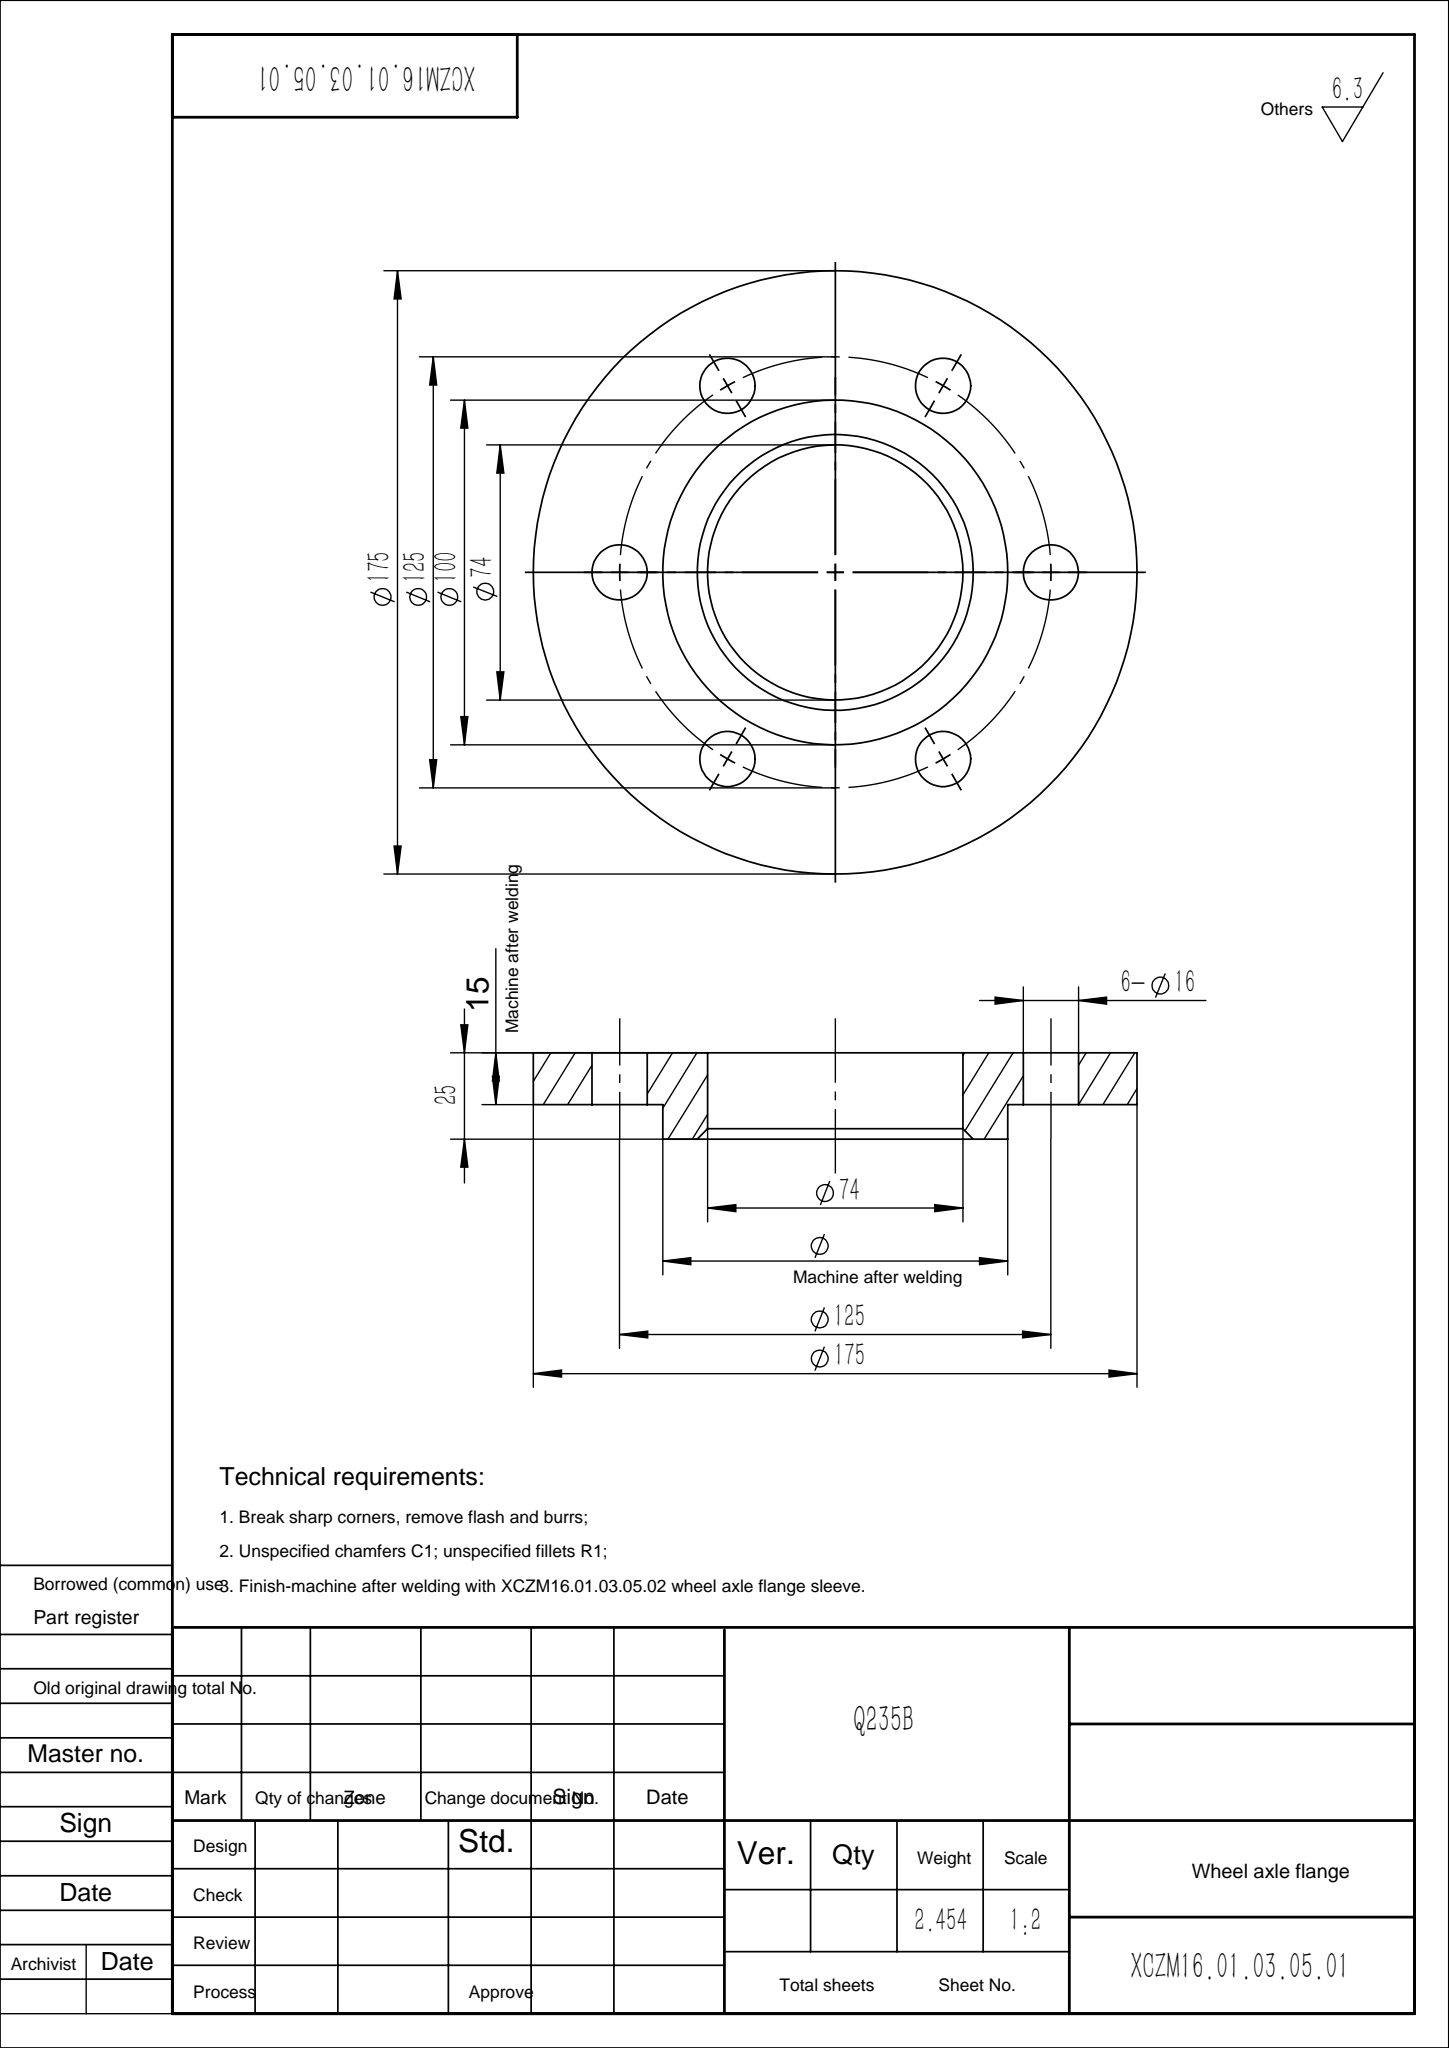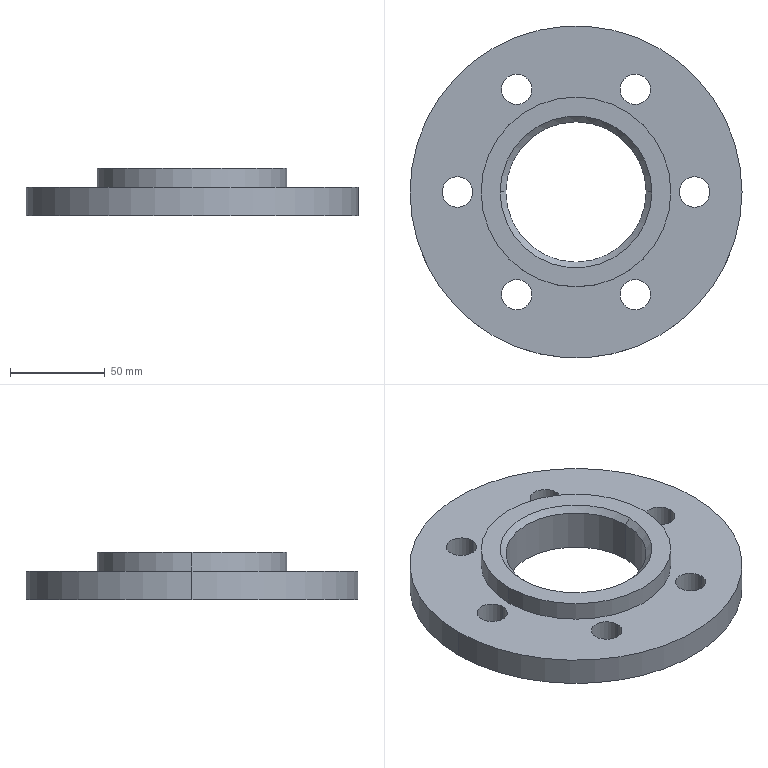Part | SolidWorks | features ICE 2, Chamfer 1, Extrusion 1, HoleWzd 1 | 1 solid | 23 faces | box 175 x 175 x 25 mm | volume 312641 mm3 | cylinder 18 | plane 3 | cone 2 | commonest cylinder face diameters 16 x12 74 x2 100 x2 175 x2
STEP:
#1=CARTESIAN_POINT('',(-37.,0.,7.));
#2=VERTEX_POINT('',#1);
#3=CARTESIAN_POINT('',(37.,0.,7.));
#4=VERTEX_POINT('',#3);
#5=CARTESIAN_POINT('',(0.,0.,7.));
#6=DIRECTION('',(0.,0.,1.));
#7=DIRECTION('',(1.,0.,0.));
#8=AXIS2_PLACEMENT_3D('',#5,#6,#7);
#9=CIRCLE('',#8,37.);
#10=EDGE_CURVE('',#2,#4,#9,.T.);
#11=ORIENTED_EDGE('',*,*,#10,.F.);
#12=CARTESIAN_POINT('',(-40.,0.,10.));
#13=VERTEX_POINT('',#12);
#14=CARTESIAN_POINT('',(-37.,0.,7.));
#15=DIRECTION('',(-0.7071,0.,0.7071));
#16=VECTOR('',#15,1000.);
#17=LINE('',#14,#16);
#18=EDGE_CURVE('',#2,#13,#17,.T.);
#19=ORIENTED_EDGE('',*,*,#18,.T.);
#20=CARTESIAN_POINT('',(40.,0.,10.));
#21=VERTEX_POINT('',#20);
#22=CARTESIAN_POINT('',(0.,0.,10.));
#23=DIRECTION('',(0.,0.,-1.));
#24=DIRECTION('',(1.,0.,0.));
#25=AXIS2_PLACEMENT_3D('',#22,#23,#24);
#26=CIRCLE('',#25,40.);
#27=EDGE_CURVE('',#21,#13,#26,.T.);
#28=ORIENTED_EDGE('',*,*,#27,.F.);
#29=CARTESIAN_POINT('',(37.,0.,7.));
#30=DIRECTION('',(0.7071,0.,0.7071));
#31=VECTOR('',#30,1000.);
#32=LINE('',#29,#31);
#33=EDGE_CURVE('',#4,#21,#32,.T.);
#34=ORIENTED_EDGE('',*,*,#33,.F.);
#35=EDGE_LOOP('',(#11,#19,#28,#34));
#36=FACE_OUTER_BOUND('',#35,.T.);
#37=CARTESIAN_POINT('',(0.,0.,7.));
#38=DIRECTION('',(0.,0.,1.));
#39=DIRECTION('',(1.,0.,0.));
#40=AXIS2_PLACEMENT_3D('',#37,#38,#39);
#41=CONICAL_SURFACE('',#40,37.,0.7854);
#42=ADVANCED_FACE('',(#36),#41,.F.);
#43=CARTESIAN_POINT('',(54.5,0.,-15.));
#44=VERTEX_POINT('',#43);
#45=CARTESIAN_POINT('',(70.5,0.,-15.));
#46=VERTEX_POINT('',#45);
#47=CARTESIAN_POINT('',(62.5,0.,-15.));
#48=DIRECTION('',(0.,0.,1.));
#49=DIRECTION('',(1.,0.,0.));
#50=AXIS2_PLACEMENT_3D('',#47,#48,#49);
#51=CIRCLE('',#50,8.);
#52=EDGE_CURVE('',#44,#46,#51,.T.);
#53=ORIENTED_EDGE('',*,*,#52,.F.);
#54=CARTESIAN_POINT('',(54.5,0.,0.));
#55=VERTEX_POINT('',#54);
#56=CARTESIAN_POINT('',(54.5,0.,0.));
#57=DIRECTION('',(0.,0.,1.));
#58=VECTOR('',#57,1000.);
#59=LINE('',#56,#58);
#60=EDGE_CURVE('',#44,#55,#59,.T.);
#61=ORIENTED_EDGE('',*,*,#60,.T.);
#62=CARTESIAN_POINT('',(70.5,0.,0.));
#63=VERTEX_POINT('',#62);
#64=CARTESIAN_POINT('',(62.5,0.,0.));
#65=DIRECTION('',(0.,0.,1.));
#66=DIRECTION('',(1.,0.,0.));
#67=AXIS2_PLACEMENT_3D('',#64,#65,#66);
#68=CIRCLE('',#67,8.);
#69=EDGE_CURVE('',#55,#63,#68,.T.);
#70=ORIENTED_EDGE('',*,*,#69,.T.);
#71=CARTESIAN_POINT('',(70.5,0.,0.));
#72=DIRECTION('',(0.,0.,1.));
#73=VECTOR('',#72,1000.);
#74=LINE('',#71,#73);
#75=EDGE_CURVE('',#46,#63,#74,.T.);
#76=ORIENTED_EDGE('',*,*,#75,.F.);
#77=EDGE_LOOP('',(#53,#61,#70,#76));
#78=FACE_OUTER_BOUND('',#77,.T.);
#79=CARTESIAN_POINT('',(62.5,0.,0.));
#80=DIRECTION('',(0.,0.,1.));
#81=DIRECTION('',(1.,0.,0.));
#82=AXIS2_PLACEMENT_3D('',#79,#80,#81);
#83=CYLINDRICAL_SURFACE('',#82,8.);
#84=ADVANCED_FACE('',(#78),#83,.F.);
#85=CARTESIAN_POINT('',(23.25,-54.127,-15.));
#86=VERTEX_POINT('',#85);
#87=CARTESIAN_POINT('',(39.25,-54.127,-15.));
#88=VERTEX_POINT('',#87);
#89=CARTESIAN_POINT('',(31.25,-54.127,-15.));
#90=DIRECTION('',(0.,0.,1.));
#91=DIRECTION('',(1.,0.,0.));
#92=AXIS2_PLACEMENT_3D('',#89,#90,#91);
#93=CIRCLE('',#92,8.);
#94=EDGE_CURVE('',#86,#88,#93,.T.);
#95=ORIENTED_EDGE('',*,*,#94,.F.);
#96=CARTESIAN_POINT('',(23.25,-54.127,0.));
#97=VERTEX_POINT('',#96);
#98=CARTESIAN_POINT('',(23.25,-54.127,0.));
#99=DIRECTION('',(0.,0.,1.));
#100=VECTOR('',#99,1000.);
#101=LINE('',#98,#100);
#102=EDGE_CURVE('',#86,#97,#101,.T.);
#103=ORIENTED_EDGE('',*,*,#102,.T.);
#104=CARTESIAN_POINT('',(39.25,-54.127,0.));
#105=VERTEX_POINT('',#104);
#106=CARTESIAN_POINT('',(31.25,-54.127,0.));
#107=DIRECTION('',(0.,0.,1.));
#108=DIRECTION('',(1.,0.,0.));
#109=AXIS2_PLACEMENT_3D('',#106,#107,#108);
#110=CIRCLE('',#109,8.);
#111=EDGE_CURVE('',#97,#105,#110,.T.);
#112=ORIENTED_EDGE('',*,*,#111,.T.);
#113=CARTESIAN_POINT('',(39.25,-54.127,0.));
#114=DIRECTION('',(0.,0.,1.));
#115=VECTOR('',#114,1000.);
#116=LINE('',#113,#115);
#117=EDGE_CURVE('',#88,#105,#116,.T.);
#118=ORIENTED_EDGE('',*,*,#117,.F.);
#119=EDGE_LOOP('',(#95,#103,#112,#118));
#120=FACE_OUTER_BOUND('',#119,.T.);
#121=CARTESIAN_POINT('',(31.25,-54.127,0.));
#122=DIRECTION('',(0.,0.,1.));
#123=DIRECTION('',(1.,0.,0.));
#124=AXIS2_PLACEMENT_3D('',#121,#122,#123);
#125=CYLINDRICAL_SURFACE('',#124,8.);
#126=ADVANCED_FACE('',(#120),#125,.F.);
#127=CARTESIAN_POINT('',(-39.25,-54.127,-15.));
#128=VERTEX_POINT('',#127);
#129=CARTESIAN_POINT('',(-23.25,-54.127,-15.));
#130=VERTEX_POINT('',#129);
#131=CARTESIAN_POINT('',(-31.25,-54.127,-15.));
#132=DIRECTION('',(0.,0.,1.));
#133=DIRECTION('',(1.,0.,0.));
#134=AXIS2_PLACEMENT_3D('',#131,#132,#133);
#135=CIRCLE('',#134,8.);
#136=EDGE_CURVE('',#128,#130,#135,.T.);
#137=ORIENTED_EDGE('',*,*,#136,.F.);
#138=CARTESIAN_POINT('',(-39.25,-54.127,0.));
#139=VERTEX_POINT('',#138);
#140=CARTESIAN_POINT('',(-39.25,-54.127,0.));
#141=DIRECTION('',(0.,0.,1.));
#142=VECTOR('',#141,1000.);
#143=LINE('',#140,#142);
#144=EDGE_CURVE('',#128,#139,#143,.T.);
#145=ORIENTED_EDGE('',*,*,#144,.T.);
#146=CARTESIAN_POINT('',(-23.25,-54.127,0.));
#147=VERTEX_POINT('',#146);
#148=CARTESIAN_POINT('',(-31.25,-54.127,0.));
#149=DIRECTION('',(0.,0.,1.));
#150=DIRECTION('',(1.,0.,0.));
#151=AXIS2_PLACEMENT_3D('',#148,#149,#150);
#152=CIRCLE('',#151,8.);
#153=EDGE_CURVE('',#139,#147,#152,.T.);
#154=ORIENTED_EDGE('',*,*,#153,.T.);
#155=CARTESIAN_POINT('',(-23.25,-54.127,0.));
#156=DIRECTION('',(0.,0.,1.));
#157=VECTOR('',#156,1000.);
#158=LINE('',#155,#157);
#159=EDGE_CURVE('',#130,#147,#158,.T.);
#160=ORIENTED_EDGE('',*,*,#159,.F.);
#161=EDGE_LOOP('',(#137,#145,#154,#160));
#162=FACE_OUTER_BOUND('',#161,.T.);
#163=CARTESIAN_POINT('',(-31.25,-54.127,0.));
#164=DIRECTION('',(0.,0.,1.));
#165=DIRECTION('',(1.,0.,0.));
#166=AXIS2_PLACEMENT_3D('',#163,#164,#165);
#167=CYLINDRICAL_SURFACE('',#166,8.);
#168=ADVANCED_FACE('',(#162),#167,.F.);
#169=CARTESIAN_POINT('',(-70.5,0.,-15.));
#170=VERTEX_POINT('',#169);
#171=CARTESIAN_POINT('',(-54.5,0.,-15.));
#172=VERTEX_POINT('',#171);
#173=CARTESIAN_POINT('',(-62.5,0.,-15.));
#174=DIRECTION('',(0.,0.,1.));
#175=DIRECTION('',(1.,0.,0.));
#176=AXIS2_PLACEMENT_3D('',#173,#174,#175);
#177=CIRCLE('',#176,8.);
#178=EDGE_CURVE('',#170,#172,#177,.T.);
#179=ORIENTED_EDGE('',*,*,#178,.F.);
#180=CARTESIAN_POINT('',(-70.5,0.,0.));
#181=VERTEX_POINT('',#180);
#182=CARTESIAN_POINT('',(-70.5,0.,0.));
#183=DIRECTION('',(0.,0.,1.));
#184=VECTOR('',#183,1000.);
#185=LINE('',#182,#184);
#186=EDGE_CURVE('',#170,#181,#185,.T.);
#187=ORIENTED_EDGE('',*,*,#186,.T.);
#188=CARTESIAN_POINT('',(-54.5,0.,0.));
#189=VERTEX_POINT('',#188);
#190=CARTESIAN_POINT('',(-62.5,0.,0.));
#191=DIRECTION('',(0.,0.,1.));
#192=DIRECTION('',(1.,0.,0.));
#193=AXIS2_PLACEMENT_3D('',#190,#191,#192);
#194=CIRCLE('',#193,8.);
#195=EDGE_CURVE('',#181,#189,#194,.T.);
#196=ORIENTED_EDGE('',*,*,#195,.T.);
#197=CARTESIAN_POINT('',(-54.5,0.,0.));
#198=DIRECTION('',(0.,0.,1.));
#199=VECTOR('',#198,1000.);
#200=LINE('',#197,#199);
#201=EDGE_CURVE('',#172,#189,#200,.T.);
#202=ORIENTED_EDGE('',*,*,#201,.F.);
#203=EDGE_LOOP('',(#179,#187,#196,#202));
#204=FACE_OUTER_BOUND('',#203,.T.);
#205=CARTESIAN_POINT('',(-62.5,0.,0.));
#206=DIRECTION('',(0.,0.,1.));
#207=DIRECTION('',(1.,0.,0.));
#208=AXIS2_PLACEMENT_3D('',#205,#206,#207);
#209=CYLINDRICAL_SURFACE('',#208,8.);
#210=ADVANCED_FACE('',(#204),#209,.F.);
#211=CARTESIAN_POINT('',(-39.25,54.127,-15.));
#212=VERTEX_POINT('',#211);
#213=CARTESIAN_POINT('',(-23.25,54.127,-15.));
#214=VERTEX_POINT('',#213);
#215=CARTESIAN_POINT('',(-31.25,54.127,-15.));
#216=DIRECTION('',(0.,0.,1.));
#217=DIRECTION('',(1.,0.,0.));
#218=AXIS2_PLACEMENT_3D('',#215,#216,#217);
#219=CIRCLE('',#218,8.);
#220=EDGE_CURVE('',#212,#214,#219,.T.);
#221=ORIENTED_EDGE('',*,*,#220,.F.);
#222=CARTESIAN_POINT('',(-39.25,54.127,0.));
#223=VERTEX_POINT('',#222);
#224=CARTESIAN_POINT('',(-39.25,54.127,0.));
#225=DIRECTION('',(0.,0.,1.));
#226=VECTOR('',#225,1000.);
#227=LINE('',#224,#226);
#228=EDGE_CURVE('',#212,#223,#227,.T.);
#229=ORIENTED_EDGE('',*,*,#228,.T.);
#230=CARTESIAN_POINT('',(-23.25,54.127,0.));
#231=VERTEX_POINT('',#230);
#232=CARTESIAN_POINT('',(-31.25,54.127,0.));
#233=DIRECTION('',(0.,0.,1.));
#234=DIRECTION('',(1.,0.,0.));
#235=AXIS2_PLACEMENT_3D('',#232,#233,#234);
#236=CIRCLE('',#235,8.);
#237=EDGE_CURVE('',#223,#231,#236,.T.);
#238=ORIENTED_EDGE('',*,*,#237,.T.);
#239=CARTESIAN_POINT('',(-23.25,54.127,0.));
#240=DIRECTION('',(0.,0.,1.));
#241=VECTOR('',#240,1000.);
#242=LINE('',#239,#241);
#243=EDGE_CURVE('',#214,#231,#242,.T.);
#244=ORIENTED_EDGE('',*,*,#243,.F.);
#245=EDGE_LOOP('',(#221,#229,#238,#244));
#246=FACE_OUTER_BOUND('',#245,.T.);
#247=CARTESIAN_POINT('',(-31.25,54.127,0.));
#248=DIRECTION('',(0.,0.,1.));
#249=DIRECTION('',(1.,0.,0.));
#250=AXIS2_PLACEMENT_3D('',#247,#248,#249);
#251=CYLINDRICAL_SURFACE('',#250,8.);
#252=ADVANCED_FACE('',(#246),#251,.F.);
#253=CARTESIAN_POINT('',(23.25,54.127,-15.));
#254=VERTEX_POINT('',#253);
#255=CARTESIAN_POINT('',(39.25,54.127,-15.));
#256=VERTEX_POINT('',#255);
#257=CARTESIAN_POINT('',(31.25,54.127,-15.));
#258=DIRECTION('',(0.,0.,1.));
#259=DIRECTION('',(1.,0.,0.));
#260=AXIS2_PLACEMENT_3D('',#257,#258,#259);
#261=CIRCLE('',#260,8.);
#262=EDGE_CURVE('',#254,#256,#261,.T.);
#263=ORIENTED_EDGE('',*,*,#262,.F.);
#264=CARTESIAN_POINT('',(23.25,54.127,0.));
#265=VERTEX_POINT('',#264);
#266=CARTESIAN_POINT('',(23.25,54.127,0.));
#267=DIRECTION('',(0.,0.,1.));
#268=VECTOR('',#267,1000.);
#269=LINE('',#266,#268);
#270=EDGE_CURVE('',#254,#265,#269,.T.);
#271=ORIENTED_EDGE('',*,*,#270,.T.);
#272=CARTESIAN_POINT('',(39.25,54.127,0.));
#273=VERTEX_POINT('',#272);
#274=CARTESIAN_POINT('',(31.25,54.127,0.));
#275=DIRECTION('',(0.,0.,1.));
#276=DIRECTION('',(1.,0.,0.));
#277=AXIS2_PLACEMENT_3D('',#274,#275,#276);
#278=CIRCLE('',#277,8.);
#279=EDGE_CURVE('',#265,#273,#278,.T.);
#280=ORIENTED_EDGE('',*,*,#279,.T.);
#281=CARTESIAN_POINT('',(39.25,54.127,0.));
#282=DIRECTION('',(0.,0.,1.));
#283=VECTOR('',#282,1000.);
#284=LINE('',#281,#283);
#285=EDGE_CURVE('',#256,#273,#284,.T.);
#286=ORIENTED_EDGE('',*,*,#285,.F.);
#287=EDGE_LOOP('',(#263,#271,#280,#286));
#288=FACE_OUTER_BOUND('',#287,.T.);
#289=CARTESIAN_POINT('',(31.25,54.127,0.));
#290=DIRECTION('',(0.,0.,1.));
#291=DIRECTION('',(1.,0.,0.));
#292=AXIS2_PLACEMENT_3D('',#289,#290,#291);
#293=CYLINDRICAL_SURFACE('',#292,8.);
#294=ADVANCED_FACE('',(#288),#293,.F.);
#295=CARTESIAN_POINT('',(37.,0.,-15.));
#296=VERTEX_POINT('',#295);
#297=CARTESIAN_POINT('',(-37.,0.,-15.));
#298=VERTEX_POINT('',#297);
#299=CARTESIAN_POINT('',(0.,0.,-15.));
#300=DIRECTION('',(0.,0.,-1.));
#301=DIRECTION('',(1.,0.,0.));
#302=AXIS2_PLACEMENT_3D('',#299,#300,#301);
#303=CIRCLE('',#302,37.);
#304=EDGE_CURVE('',#296,#298,#303,.T.);
#305=ORIENTED_EDGE('',*,*,#304,.T.);
#306=CARTESIAN_POINT('',(-37.,0.,-15.001));
#307=DIRECTION('',(0.,0.,1.));
#308=VECTOR('',#307,1000.);
#309=LINE('',#306,#308);
#310=EDGE_CURVE('',#298,#2,#309,.T.);
#311=ORIENTED_EDGE('',*,*,#310,.T.);
#312=ORIENTED_EDGE('',*,*,#10,.T.);
#313=CARTESIAN_POINT('',(37.,0.,-15.001));
#314=DIRECTION('',(0.,0.,1.));
#315=VECTOR('',#314,1000.);
#316=LINE('',#313,#315);
#317=EDGE_CURVE('',#296,#4,#316,.T.);
#318=ORIENTED_EDGE('',*,*,#317,.F.);
#319=EDGE_LOOP('',(#305,#311,#312,#318));
#320=FACE_OUTER_BOUND('',#319,.T.);
#321=CARTESIAN_POINT('',(0.,0.,-15.001));
#322=DIRECTION('',(0.,0.,1.));
#323=DIRECTION('',(1.,0.,0.));
#324=AXIS2_PLACEMENT_3D('',#321,#322,#323);
#325=CYLINDRICAL_SURFACE('',#324,37.);
#326=ADVANCED_FACE('',(#320),#325,.F.);
#327=CARTESIAN_POINT('',(87.5,0.,-15.));
#328=VERTEX_POINT('',#327);
#329=CARTESIAN_POINT('',(-87.5,0.,-15.));
#330=VERTEX_POINT('',#329);
#331=CARTESIAN_POINT('',(0.,0.,-15.));
#332=DIRECTION('',(0.,0.,1.));
#333=DIRECTION('',(1.,0.,0.));
#334=AXIS2_PLACEMENT_3D('',#331,#332,#333);
#335=CIRCLE('',#334,87.5);
#336=EDGE_CURVE('',#328,#330,#335,.T.);
#337=ORIENTED_EDGE('',*,*,#336,.T.);
#338=CARTESIAN_POINT('',(-87.5,0.,0.));
#339=VERTEX_POINT('',#338);
#340=CARTESIAN_POINT('',(-87.5,0.,-15.));
#341=DIRECTION('',(0.,0.,1.));
#342=VECTOR('',#341,1000.);
#343=LINE('',#340,#342);
#344=EDGE_CURVE('',#330,#339,#343,.T.);
#345=ORIENTED_EDGE('',*,*,#344,.T.);
#346=CARTESIAN_POINT('',(87.5,0.,0.));
#347=VERTEX_POINT('',#346);
#348=CARTESIAN_POINT('',(0.,0.,0.));
#349=DIRECTION('',(0.,0.,1.));
#350=DIRECTION('',(1.,0.,0.));
#351=AXIS2_PLACEMENT_3D('',#348,#349,#350);
#352=CIRCLE('',#351,87.5);
#353=EDGE_CURVE('',#347,#339,#352,.T.);
#354=ORIENTED_EDGE('',*,*,#353,.F.);
#355=CARTESIAN_POINT('',(87.5,0.,-15.));
#356=DIRECTION('',(0.,0.,1.));
#357=VECTOR('',#356,1000.);
#358=LINE('',#355,#357);
#359=EDGE_CURVE('',#328,#347,#358,.T.);
#360=ORIENTED_EDGE('',*,*,#359,.F.);
#361=EDGE_LOOP('',(#337,#345,#354,#360));
#362=FACE_OUTER_BOUND('',#361,.T.);
#363=CARTESIAN_POINT('',(0.,0.,-15.));
#364=DIRECTION('',(0.,0.,1.));
#365=DIRECTION('',(1.,0.,0.));
#366=AXIS2_PLACEMENT_3D('',#363,#364,#365);
#367=CYLINDRICAL_SURFACE('',#366,87.5);
#368=ADVANCED_FACE('',(#362),#367,.T.);
#369=CARTESIAN_POINT('',(50.,0.,10.));
#370=VERTEX_POINT('',#369);
#371=CARTESIAN_POINT('',(-50.,0.,10.));
#372=VERTEX_POINT('',#371);
#373=CARTESIAN_POINT('',(0.,0.,10.));
#374=DIRECTION('',(0.,0.,1.));
#375=DIRECTION('',(1.,0.,0.));
#376=AXIS2_PLACEMENT_3D('',#373,#374,#375);
#377=CIRCLE('',#376,50.);
#378=EDGE_CURVE('',#370,#372,#377,.T.);
#379=ORIENTED_EDGE('',*,*,#378,.F.);
#380=CARTESIAN_POINT('',(50.,0.,0.));
#381=VERTEX_POINT('',#380);
#382=CARTESIAN_POINT('',(50.,0.,10.));
#383=DIRECTION('',(0.,0.,-1.));
#384=VECTOR('',#383,1000.);
#385=LINE('',#382,#384);
#386=EDGE_CURVE('',#370,#381,#385,.T.);
#387=ORIENTED_EDGE('',*,*,#386,.T.);
#388=CARTESIAN_POINT('',(-50.,0.,0.));
#389=VERTEX_POINT('',#388);
#390=CARTESIAN_POINT('',(0.,0.,0.));
#391=DIRECTION('',(0.,0.,1.));
#392=DIRECTION('',(1.,0.,0.));
#393=AXIS2_PLACEMENT_3D('',#390,#391,#392);
#394=CIRCLE('',#393,50.);
#395=EDGE_CURVE('',#381,#389,#394,.T.);
#396=ORIENTED_EDGE('',*,*,#395,.T.);
#397=CARTESIAN_POINT('',(-50.,0.,10.));
#398=DIRECTION('',(0.,0.,-1.));
#399=VECTOR('',#398,1000.);
#400=LINE('',#397,#399);
#401=EDGE_CURVE('',#372,#389,#400,.T.);
#402=ORIENTED_EDGE('',*,*,#401,.F.);
#403=EDGE_LOOP('',(#379,#387,#396,#402));
#404=FACE_OUTER_BOUND('',#403,.T.);
#405=CARTESIAN_POINT('',(0.,0.,10.));
#406=DIRECTION('',(0.,0.,-1.));
#407=DIRECTION('',(-1.,0.,0.));
#408=AXIS2_PLACEMENT_3D('',#405,#406,#407);
#409=CYLINDRICAL_SURFACE('',#408,50.);
#410=ADVANCED_FACE('',(#404),#409,.T.);
#411=ORIENTED_EDGE('',*,*,#386,.F.);
#412=CARTESIAN_POINT('',(0.,0.,10.));
#413=DIRECTION('',(0.,0.,1.));
#414=DIRECTION('',(1.,0.,0.));
#415=AXIS2_PLACEMENT_3D('',#412,#413,#414);
#416=CIRCLE('',#415,50.);
#417=EDGE_CURVE('',#372,#370,#416,.T.);
#418=ORIENTED_EDGE('',*,*,#417,.F.);
#419=ORIENTED_EDGE('',*,*,#401,.T.);
#420=CARTESIAN_POINT('',(0.,0.,0.));
#421=DIRECTION('',(0.,0.,1.));
#422=DIRECTION('',(1.,0.,0.));
#423=AXIS2_PLACEMENT_3D('',#420,#421,#422);
#424=CIRCLE('',#423,50.);
#425=EDGE_CURVE('',#389,#381,#424,.T.);
#426=ORIENTED_EDGE('',*,*,#425,.T.);
#427=EDGE_LOOP('',(#411,#418,#419,#426));
#428=FACE_OUTER_BOUND('',#427,.T.);
#429=CARTESIAN_POINT('',(0.,0.,10.));
#430=DIRECTION('',(0.,0.,-1.));
#431=DIRECTION('',(-1.,0.,0.));
#432=AXIS2_PLACEMENT_3D('',#429,#430,#431);
#433=CYLINDRICAL_SURFACE('',#432,50.);
#434=ADVANCED_FACE('',(#428),#433,.T.);
#435=ORIENTED_EDGE('',*,*,#27,.T.);
#436=CARTESIAN_POINT('',(0.,0.,10.));
#437=DIRECTION('',(0.,0.,-1.));
#438=DIRECTION('',(1.,0.,0.));
#439=AXIS2_PLACEMENT_3D('',#436,#437,#438);
#440=CIRCLE('',#439,40.);
#441=EDGE_CURVE('',#13,#21,#440,.T.);
#442=ORIENTED_EDGE('',*,*,#441,.T.);
#443=EDGE_LOOP('',(#435,#442));
#444=FACE_BOUND('',#443,.T.);
#445=ORIENTED_EDGE('',*,*,#417,.T.);
#446=ORIENTED_EDGE('',*,*,#378,.T.);
#447=EDGE_LOOP('',(#445,#446));
#448=FACE_OUTER_BOUND('',#447,.T.);
#449=CARTESIAN_POINT('',(0.,0.,10.));
#450=DIRECTION('',(0.,0.,1.));
#451=DIRECTION('',(1.,0.,0.));
#452=AXIS2_PLACEMENT_3D('',#449,#450,#451);
#453=PLANE('',#452);
#454=ADVANCED_FACE('',(#444,#448),#453,.T.);
#455=ORIENTED_EDGE('',*,*,#344,.F.);
#456=CARTESIAN_POINT('',(0.,0.,-15.));
#457=DIRECTION('',(0.,0.,1.));
#458=DIRECTION('',(1.,0.,0.));
#459=AXIS2_PLACEMENT_3D('',#456,#457,#458);
#460=CIRCLE('',#459,87.5);
#461=EDGE_CURVE('',#330,#328,#460,.T.);
#462=ORIENTED_EDGE('',*,*,#461,.T.);
#463=ORIENTED_EDGE('',*,*,#359,.T.);
#464=CARTESIAN_POINT('',(0.,0.,0.));
#465=DIRECTION('',(0.,0.,1.));
#466=DIRECTION('',(1.,0.,0.));
#467=AXIS2_PLACEMENT_3D('',#464,#465,#466);
#468=CIRCLE('',#467,87.5);
#469=EDGE_CURVE('',#339,#347,#468,.T.);
#470=ORIENTED_EDGE('',*,*,#469,.F.);
#471=EDGE_LOOP('',(#455,#462,#463,#470));
#472=FACE_OUTER_BOUND('',#471,.T.);
#473=CARTESIAN_POINT('',(0.,0.,-15.));
#474=DIRECTION('',(0.,0.,1.));
#475=DIRECTION('',(1.,0.,0.));
#476=AXIS2_PLACEMENT_3D('',#473,#474,#475);
#477=CYLINDRICAL_SURFACE('',#476,87.5);
#478=ADVANCED_FACE('',(#472),#477,.T.);
#479=CARTESIAN_POINT('',(62.5,0.,-15.));
#480=DIRECTION('',(0.,0.,1.));
#481=DIRECTION('',(1.,0.,0.));
#482=AXIS2_PLACEMENT_3D('',#479,#480,#481);
#483=CIRCLE('',#482,8.);
#484=EDGE_CURVE('',#46,#44,#483,.T.);
#485=ORIENTED_EDGE('',*,*,#484,.T.);
#486=ORIENTED_EDGE('',*,*,#52,.T.);
#487=EDGE_LOOP('',(#485,#486));
#488=FACE_BOUND('',#487,.T.);
#489=CARTESIAN_POINT('',(31.25,-54.127,-15.));
#490=DIRECTION('',(0.,0.,1.));
#491=DIRECTION('',(1.,0.,0.));
#492=AXIS2_PLACEMENT_3D('',#489,#490,#491);
#493=CIRCLE('',#492,8.);
#494=EDGE_CURVE('',#88,#86,#493,.T.);
#495=ORIENTED_EDGE('',*,*,#494,.T.);
#496=ORIENTED_EDGE('',*,*,#94,.T.);
#497=EDGE_LOOP('',(#495,#496));
#498=FACE_BOUND('',#497,.T.);
#499=CARTESIAN_POINT('',(-31.25,-54.127,-15.));
#500=DIRECTION('',(0.,0.,1.));
#501=DIRECTION('',(1.,0.,0.));
#502=AXIS2_PLACEMENT_3D('',#499,#500,#501);
#503=CIRCLE('',#502,8.);
#504=EDGE_CURVE('',#130,#128,#503,.T.);
#505=ORIENTED_EDGE('',*,*,#504,.T.);
#506=ORIENTED_EDGE('',*,*,#136,.T.);
#507=EDGE_LOOP('',(#505,#506));
#508=FACE_BOUND('',#507,.T.);
#509=CARTESIAN_POINT('',(-62.5,0.,-15.));
#510=DIRECTION('',(0.,0.,1.));
#511=DIRECTION('',(1.,0.,0.));
#512=AXIS2_PLACEMENT_3D('',#509,#510,#511);
#513=CIRCLE('',#512,8.);
#514=EDGE_CURVE('',#172,#170,#513,.T.);
#515=ORIENTED_EDGE('',*,*,#514,.T.);
#516=ORIENTED_EDGE('',*,*,#178,.T.);
#517=EDGE_LOOP('',(#515,#516));
#518=FACE_BOUND('',#517,.T.);
#519=CARTESIAN_POINT('',(-31.25,54.127,-15.));
#520=DIRECTION('',(0.,0.,1.));
#521=DIRECTION('',(1.,0.,0.));
#522=AXIS2_PLACEMENT_3D('',#519,#520,#521);
#523=CIRCLE('',#522,8.);
#524=EDGE_CURVE('',#214,#212,#523,.T.);
#525=ORIENTED_EDGE('',*,*,#524,.T.);
#526=ORIENTED_EDGE('',*,*,#220,.T.);
#527=EDGE_LOOP('',(#525,#526));
#528=FACE_BOUND('',#527,.T.);
#529=CARTESIAN_POINT('',(31.25,54.127,-15.));
#530=DIRECTION('',(0.,0.,1.));
#531=DIRECTION('',(1.,0.,0.));
#532=AXIS2_PLACEMENT_3D('',#529,#530,#531);
#533=CIRCLE('',#532,8.);
#534=EDGE_CURVE('',#256,#254,#533,.T.);
#535=ORIENTED_EDGE('',*,*,#534,.T.);
#536=ORIENTED_EDGE('',*,*,#262,.T.);
#537=EDGE_LOOP('',(#535,#536));
#538=FACE_BOUND('',#537,.T.);
#539=ORIENTED_EDGE('',*,*,#304,.F.);
#540=CARTESIAN_POINT('',(0.,0.,-15.));
#541=DIRECTION('',(0.,0.,-1.));
#542=DIRECTION('',(1.,0.,0.));
#543=AXIS2_PLACEMENT_3D('',#540,#541,#542);
#544=CIRCLE('',#543,37.);
#545=EDGE_CURVE('',#298,#296,#544,.T.);
#546=ORIENTED_EDGE('',*,*,#545,.F.);
#547=EDGE_LOOP('',(#539,#546));
#548=FACE_BOUND('',#547,.T.);
#549=ORIENTED_EDGE('',*,*,#336,.F.);
#550=ORIENTED_EDGE('',*,*,#461,.F.);
#551=EDGE_LOOP('',(#549,#550));
#552=FACE_OUTER_BOUND('',#551,.T.);
#553=CARTESIAN_POINT('',(0.,0.,-15.));
#554=DIRECTION('',(0.,0.,1.));
#555=DIRECTION('',(1.,0.,0.));
#556=AXIS2_PLACEMENT_3D('',#553,#554,#555);
#557=PLANE('',#556);
#558=ADVANCED_FACE('',(#488,#498,#508,#518,#528,#538,#548,#552),#557,.F.);
#559=CARTESIAN_POINT('',(62.5,0.,0.));
#560=DIRECTION('',(0.,0.,1.));
#561=DIRECTION('',(1.,0.,0.));
#562=AXIS2_PLACEMENT_3D('',#559,#560,#561);
#563=CIRCLE('',#562,8.);
#564=EDGE_CURVE('',#63,#55,#563,.T.);
#565=ORIENTED_EDGE('',*,*,#564,.F.);
#566=ORIENTED_EDGE('',*,*,#69,.F.);
#567=EDGE_LOOP('',(#565,#566));
#568=FACE_BOUND('',#567,.T.);
#569=CARTESIAN_POINT('',(31.25,-54.127,0.));
#570=DIRECTION('',(0.,0.,1.));
#571=DIRECTION('',(1.,0.,0.));
#572=AXIS2_PLACEMENT_3D('',#569,#570,#571);
#573=CIRCLE('',#572,8.);
#574=EDGE_CURVE('',#105,#97,#573,.T.);
#575=ORIENTED_EDGE('',*,*,#574,.F.);
#576=ORIENTED_EDGE('',*,*,#111,.F.);
#577=EDGE_LOOP('',(#575,#576));
#578=FACE_BOUND('',#577,.T.);
#579=CARTESIAN_POINT('',(-31.25,-54.127,0.));
#580=DIRECTION('',(0.,0.,1.));
#581=DIRECTION('',(1.,0.,0.));
#582=AXIS2_PLACEMENT_3D('',#579,#580,#581);
#583=CIRCLE('',#582,8.);
#584=EDGE_CURVE('',#147,#139,#583,.T.);
#585=ORIENTED_EDGE('',*,*,#584,.F.);
#586=ORIENTED_EDGE('',*,*,#153,.F.);
#587=EDGE_LOOP('',(#585,#586));
#588=FACE_BOUND('',#587,.T.);
#589=CARTESIAN_POINT('',(-62.5,0.,0.));
#590=DIRECTION('',(0.,0.,1.));
#591=DIRECTION('',(1.,0.,0.));
#592=AXIS2_PLACEMENT_3D('',#589,#590,#591);
#593=CIRCLE('',#592,8.);
#594=EDGE_CURVE('',#189,#181,#593,.T.);
#595=ORIENTED_EDGE('',*,*,#594,.F.);
#596=ORIENTED_EDGE('',*,*,#195,.F.);
#597=EDGE_LOOP('',(#595,#596));
#598=FACE_BOUND('',#597,.T.);
#599=CARTESIAN_POINT('',(-31.25,54.127,0.));
#600=DIRECTION('',(0.,0.,1.));
#601=DIRECTION('',(1.,0.,0.));
#602=AXIS2_PLACEMENT_3D('',#599,#600,#601);
#603=CIRCLE('',#602,8.);
#604=EDGE_CURVE('',#231,#223,#603,.T.);
#605=ORIENTED_EDGE('',*,*,#604,.F.);
#606=ORIENTED_EDGE('',*,*,#237,.F.);
#607=EDGE_LOOP('',(#605,#606));
#608=FACE_BOUND('',#607,.T.);
#609=CARTESIAN_POINT('',(31.25,54.127,0.));
#610=DIRECTION('',(0.,0.,1.));
#611=DIRECTION('',(1.,0.,0.));
#612=AXIS2_PLACEMENT_3D('',#609,#610,#611);
#613=CIRCLE('',#612,8.);
#614=EDGE_CURVE('',#273,#265,#613,.T.);
#615=ORIENTED_EDGE('',*,*,#614,.F.);
#616=ORIENTED_EDGE('',*,*,#279,.F.);
#617=EDGE_LOOP('',(#615,#616));
#618=FACE_BOUND('',#617,.T.);
#619=ORIENTED_EDGE('',*,*,#425,.F.);
#620=ORIENTED_EDGE('',*,*,#395,.F.);
#621=EDGE_LOOP('',(#619,#620));
#622=FACE_BOUND('',#621,.T.);
#623=ORIENTED_EDGE('',*,*,#353,.T.);
#624=ORIENTED_EDGE('',*,*,#469,.T.);
#625=EDGE_LOOP('',(#623,#624));
#626=FACE_OUTER_BOUND('',#625,.T.);
#627=CARTESIAN_POINT('',(0.,0.,0.));
#628=DIRECTION('',(0.,0.,1.));
#629=DIRECTION('',(1.,0.,0.));
#630=AXIS2_PLACEMENT_3D('',#627,#628,#629);
#631=PLANE('',#630);
#632=ADVANCED_FACE('',(#568,#578,#588,#598,#608,#618,#622,#626),#631,.T.);
#633=ORIENTED_EDGE('',*,*,#310,.F.);
#634=ORIENTED_EDGE('',*,*,#545,.T.);
#635=ORIENTED_EDGE('',*,*,#317,.T.);
#636=CARTESIAN_POINT('',(0.,0.,7.));
#637=DIRECTION('',(0.,0.,1.));
#638=DIRECTION('',(1.,0.,0.));
#639=AXIS2_PLACEMENT_3D('',#636,#637,#638);
#640=CIRCLE('',#639,37.);
#641=EDGE_CURVE('',#4,#2,#640,.T.);
#642=ORIENTED_EDGE('',*,*,#641,.T.);
#643=EDGE_LOOP('',(#633,#634,#635,#642));
#644=FACE_OUTER_BOUND('',#643,.T.);
#645=CARTESIAN_POINT('',(0.,0.,-15.001));
#646=DIRECTION('',(0.,0.,1.));
#647=DIRECTION('',(1.,0.,0.));
#648=AXIS2_PLACEMENT_3D('',#645,#646,#647);
#649=CYLINDRICAL_SURFACE('',#648,37.);
#650=ADVANCED_FACE('',(#644),#649,.F.);
#651=ORIENTED_EDGE('',*,*,#270,.F.);
#652=ORIENTED_EDGE('',*,*,#534,.F.);
#653=ORIENTED_EDGE('',*,*,#285,.T.);
#654=ORIENTED_EDGE('',*,*,#614,.T.);
#655=EDGE_LOOP('',(#651,#652,#653,#654));
#656=FACE_OUTER_BOUND('',#655,.T.);
#657=CARTESIAN_POINT('',(31.25,54.127,0.));
#658=DIRECTION('',(0.,0.,1.));
#659=DIRECTION('',(1.,0.,0.));
#660=AXIS2_PLACEMENT_3D('',#657,#658,#659);
#661=CYLINDRICAL_SURFACE('',#660,8.);
#662=ADVANCED_FACE('',(#656),#661,.F.);
#663=ORIENTED_EDGE('',*,*,#228,.F.);
#664=ORIENTED_EDGE('',*,*,#524,.F.);
#665=ORIENTED_EDGE('',*,*,#243,.T.);
#666=ORIENTED_EDGE('',*,*,#604,.T.);
#667=EDGE_LOOP('',(#663,#664,#665,#666));
#668=FACE_OUTER_BOUND('',#667,.T.);
#669=CARTESIAN_POINT('',(-31.25,54.127,0.));
#670=DIRECTION('',(0.,0.,1.));
#671=DIRECTION('',(1.,0.,0.));
#672=AXIS2_PLACEMENT_3D('',#669,#670,#671);
#673=CYLINDRICAL_SURFACE('',#672,8.);
#674=ADVANCED_FACE('',(#668),#673,.F.);
#675=ORIENTED_EDGE('',*,*,#186,.F.);
#676=ORIENTED_EDGE('',*,*,#514,.F.);
#677=ORIENTED_EDGE('',*,*,#201,.T.);
#678=ORIENTED_EDGE('',*,*,#594,.T.);
#679=EDGE_LOOP('',(#675,#676,#677,#678));
#680=FACE_OUTER_BOUND('',#679,.T.);
#681=CARTESIAN_POINT('',(-62.5,0.,0.));
#682=DIRECTION('',(0.,0.,1.));
#683=DIRECTION('',(1.,0.,0.));
#684=AXIS2_PLACEMENT_3D('',#681,#682,#683);
#685=CYLINDRICAL_SURFACE('',#684,8.);
#686=ADVANCED_FACE('',(#680),#685,.F.);
#687=ORIENTED_EDGE('',*,*,#144,.F.);
#688=ORIENTED_EDGE('',*,*,#504,.F.);
#689=ORIENTED_EDGE('',*,*,#159,.T.);
#690=ORIENTED_EDGE('',*,*,#584,.T.);
#691=EDGE_LOOP('',(#687,#688,#689,#690));
#692=FACE_OUTER_BOUND('',#691,.T.);
#693=CARTESIAN_POINT('',(-31.25,-54.127,0.));
#694=DIRECTION('',(0.,0.,1.));
#695=DIRECTION('',(1.,0.,0.));
#696=AXIS2_PLACEMENT_3D('',#693,#694,#695);
#697=CYLINDRICAL_SURFACE('',#696,8.);
#698=ADVANCED_FACE('',(#692),#697,.F.);
#699=ORIENTED_EDGE('',*,*,#102,.F.);
#700=ORIENTED_EDGE('',*,*,#494,.F.);
#701=ORIENTED_EDGE('',*,*,#117,.T.);
#702=ORIENTED_EDGE('',*,*,#574,.T.);
#703=EDGE_LOOP('',(#699,#700,#701,#702));
#704=FACE_OUTER_BOUND('',#703,.T.);
#705=CARTESIAN_POINT('',(31.25,-54.127,0.));
#706=DIRECTION('',(0.,0.,1.));
#707=DIRECTION('',(1.,0.,0.));
#708=AXIS2_PLACEMENT_3D('',#705,#706,#707);
#709=CYLINDRICAL_SURFACE('',#708,8.);
#710=ADVANCED_FACE('',(#704),#709,.F.);
#711=ORIENTED_EDGE('',*,*,#60,.F.);
#712=ORIENTED_EDGE('',*,*,#484,.F.);
#713=ORIENTED_EDGE('',*,*,#75,.T.);
#714=ORIENTED_EDGE('',*,*,#564,.T.);
#715=EDGE_LOOP('',(#711,#712,#713,#714));
#716=FACE_OUTER_BOUND('',#715,.T.);
#717=CARTESIAN_POINT('',(62.5,0.,0.));
#718=DIRECTION('',(0.,0.,1.));
#719=DIRECTION('',(1.,0.,0.));
#720=AXIS2_PLACEMENT_3D('',#717,#718,#719);
#721=CYLINDRICAL_SURFACE('',#720,8.);
#722=ADVANCED_FACE('',(#716),#721,.F.);
#723=ORIENTED_EDGE('',*,*,#18,.F.);
#724=ORIENTED_EDGE('',*,*,#641,.F.);
#725=ORIENTED_EDGE('',*,*,#33,.T.);
#726=ORIENTED_EDGE('',*,*,#441,.F.);
#727=EDGE_LOOP('',(#723,#724,#725,#726));
#728=FACE_OUTER_BOUND('',#727,.T.);
#729=CARTESIAN_POINT('',(0.,0.,7.));
#730=DIRECTION('',(0.,0.,1.));
#731=DIRECTION('',(1.,0.,0.));
#732=AXIS2_PLACEMENT_3D('',#729,#730,#731);
#733=CONICAL_SURFACE('',#732,37.,0.7854);
#734=ADVANCED_FACE('',(#728),#733,.F.);
#735=CLOSED_SHELL('',(#42,#84,#126,#168,#210,#252,#294,#326,#368,#410,#434,#454,#478,#558,#632,#650,#662,#674,#686,#698,#710,#722,#734));
#736=MANIFOLD_SOLID_BREP('',#735);
#737=CARTESIAN_POINT('',(0.,0.,0.));
#738=DIRECTION('',(0.,0.,1.));
#739=DIRECTION('',(1.,0.,0.));
#740=AXIS2_PLACEMENT_3D('',#737,#738,#739);
#741=(LENGTH_UNIT()NAMED_UNIT(*)SI_UNIT(.MILLI.,.METRE.));
#742=UNCERTAINTY_MEASURE_WITH_UNIT(LENGTH_MEASURE(0.00001),#741,'','');
#743=(NAMED_UNIT(*)PLANE_ANGLE_UNIT()SI_UNIT($,.RADIAN.));
#744=(NAMED_UNIT(*)SI_UNIT($,.STERADIAN.)SOLID_ANGLE_UNIT());
#745=(GEOMETRIC_REPRESENTATION_CONTEXT(3)GLOBAL_UNCERTAINTY_ASSIGNED_CONTEXT((#742))GLOBAL_UNIT_ASSIGNED_CONTEXT((#741,#743,#744))REPRESENTATION_CONTEXT('',''));
#746=ADVANCED_BREP_SHAPE_REPRESENTATION('',(#736,#740),#745);